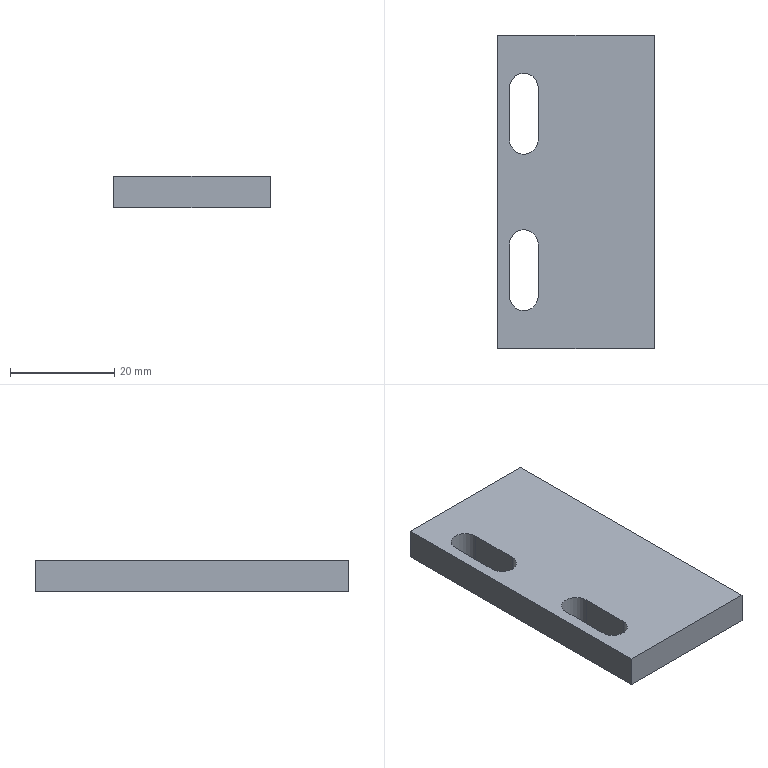Part | STEP file | 0232_208_Plate | 1 solid | 14 faces | box 30 x 60 x 6 mm | volume 9855 mm3 | plane 10 | cylinder 4 | commonest cylinder face diameters 5.5 x4
STEP:
#1=CARTESIAN_POINT('',(0.,0.,0.));
#2=DIRECTION('',(0.,0.,1.));
#3=DIRECTION('',(1.,0.,0.));
#4=AXIS2_PLACEMENT_3D('',#1,#2,#3);
#5=CARTESIAN_POINT('',(-30.,30.,0.));
#6=VERTEX_POINT('',#5);
#7=CARTESIAN_POINT('',(-30.,-30.,0.));
#8=VERTEX_POINT('',#7);
#9=CARTESIAN_POINT('',(-30.,30.,0.));
#10=DIRECTION('',(0.,-1.,0.));
#11=VECTOR('',#10,1.);
#12=LINE('',#9,#11);
#13=CARTESIAN_POINT('',(-30.,30.,6.));
#14=DIRECTION('',(1.,0.,0.));
#15=DIRECTION('',(0.,0.,-1.));
#16=AXIS2_PLACEMENT_3D('',#13,#14,#15);
#17=PLANE('',#16);
#18=CARTESIAN_POINT('',(6.,0.));
#19=DIRECTION('',(0.,-1.));
#20=VECTOR('',#19,1.);
#21=LINE('',#18,#20);
#22=(GEOMETRIC_REPRESENTATION_CONTEXT(2)PARAMETRIC_REPRESENTATION_CONTEXT()REPRESENTATION_CONTEXT('',''));
#23=DEFINITIONAL_REPRESENTATION('',(#21),#22);
#24=PCURVE('',#17,#23);
#25=CARTESIAN_POINT('',(-30.,-30.,0.));
#26=DIRECTION('',(0.,0.,1.));
#27=DIRECTION('',(1.,0.,0.));
#28=AXIS2_PLACEMENT_3D('',#25,#26,#27);
#29=PLANE('',#28);
#30=CARTESIAN_POINT('',(0.,60.));
#31=DIRECTION('',(0.,-1.));
#32=VECTOR('',#31,1.);
#33=LINE('',#30,#32);
#34=(GEOMETRIC_REPRESENTATION_CONTEXT(2)PARAMETRIC_REPRESENTATION_CONTEXT()REPRESENTATION_CONTEXT('',''));
#35=DEFINITIONAL_REPRESENTATION('',(#33),#34);
#36=PCURVE('',#29,#35);
#37=SURFACE_CURVE('',#12,(#24,#36),.PCURVE_S1.);
#38=EDGE_CURVE('',#6,#8,#37,.T.);
#39=ORIENTED_EDGE('',*,*,#38,.T.);
#40=CARTESIAN_POINT('',(-30.,-30.,6.));
#41=VERTEX_POINT('',#40);
#42=CARTESIAN_POINT('',(-30.,-30.,6.));
#43=DIRECTION('',(0.,0.,-1.));
#44=VECTOR('',#43,1.);
#45=LINE('',#42,#44);
#46=CARTESIAN_POINT('',(0.,-60.));
#47=DIRECTION('',(1.,0.));
#48=VECTOR('',#47,1.);
#49=LINE('',#46,#48);
#50=(GEOMETRIC_REPRESENTATION_CONTEXT(2)PARAMETRIC_REPRESENTATION_CONTEXT()REPRESENTATION_CONTEXT('',''));
#51=DEFINITIONAL_REPRESENTATION('',(#49),#50);
#52=PCURVE('',#17,#51);
#53=CARTESIAN_POINT('',(-30.,-30.,6.));
#54=DIRECTION('',(0.,1.,0.));
#55=DIRECTION('',(0.,0.,1.));
#56=AXIS2_PLACEMENT_3D('',#53,#54,#55);
#57=PLANE('',#56);
#58=CARTESIAN_POINT('',(0.,0.));
#59=DIRECTION('',(-1.,0.));
#60=VECTOR('',#59,1.);
#61=LINE('',#58,#60);
#62=(GEOMETRIC_REPRESENTATION_CONTEXT(2)PARAMETRIC_REPRESENTATION_CONTEXT()REPRESENTATION_CONTEXT('',''));
#63=DEFINITIONAL_REPRESENTATION('',(#61),#62);
#64=PCURVE('',#57,#63);
#65=SURFACE_CURVE('',#45,(#52,#64),.PCURVE_S1.);
#66=EDGE_CURVE('',#41,#8,#65,.T.);
#67=ORIENTED_EDGE('',*,*,#66,.F.);
#68=CARTESIAN_POINT('',(-30.,30.,6.));
#69=VERTEX_POINT('',#68);
#70=CARTESIAN_POINT('',(-30.,30.,6.));
#71=DIRECTION('',(0.,-1.,0.));
#72=VECTOR('',#71,1.);
#73=LINE('',#70,#72);
#74=CARTESIAN_POINT('',(0.,0.));
#75=DIRECTION('',(0.,-1.));
#76=VECTOR('',#75,1.);
#77=LINE('',#74,#76);
#78=(GEOMETRIC_REPRESENTATION_CONTEXT(2)PARAMETRIC_REPRESENTATION_CONTEXT()REPRESENTATION_CONTEXT('',''));
#79=DEFINITIONAL_REPRESENTATION('',(#77),#78);
#80=PCURVE('',#17,#79);
#81=CARTESIAN_POINT('',(-30.,-30.,6.));
#82=DIRECTION('',(0.,0.,1.));
#83=DIRECTION('',(1.,0.,0.));
#84=AXIS2_PLACEMENT_3D('',#81,#82,#83);
#85=PLANE('',#84);
#86=CARTESIAN_POINT('',(0.,60.));
#87=DIRECTION('',(0.,-1.));
#88=VECTOR('',#87,1.);
#89=LINE('',#86,#88);
#90=(GEOMETRIC_REPRESENTATION_CONTEXT(2)PARAMETRIC_REPRESENTATION_CONTEXT()REPRESENTATION_CONTEXT('',''));
#91=DEFINITIONAL_REPRESENTATION('',(#89),#90);
#92=PCURVE('',#85,#91);
#93=SURFACE_CURVE('',#73,(#80,#92),.PCURVE_S1.);
#94=EDGE_CURVE('',#69,#41,#93,.T.);
#95=ORIENTED_EDGE('',*,*,#94,.F.);
#96=CARTESIAN_POINT('',(-30.,30.,6.));
#97=DIRECTION('',(0.,0.,-1.));
#98=VECTOR('',#97,1.);
#99=LINE('',#96,#98);
#100=CARTESIAN_POINT('',(0.,0.));
#101=DIRECTION('',(1.,0.));
#102=VECTOR('',#101,1.);
#103=LINE('',#100,#102);
#104=(GEOMETRIC_REPRESENTATION_CONTEXT(2)PARAMETRIC_REPRESENTATION_CONTEXT()REPRESENTATION_CONTEXT('',''));
#105=DEFINITIONAL_REPRESENTATION('',(#103),#104);
#106=PCURVE('',#17,#105);
#107=CARTESIAN_POINT('',(-30.,30.,6.));
#108=DIRECTION('',(0.,-1.,0.));
#109=DIRECTION('',(0.,0.,-1.));
#110=AXIS2_PLACEMENT_3D('',#107,#108,#109);
#111=PLANE('',#110);
#112=CARTESIAN_POINT('',(0.,0.));
#113=DIRECTION('',(1.,0.));
#114=VECTOR('',#113,1.);
#115=LINE('',#112,#114);
#116=(GEOMETRIC_REPRESENTATION_CONTEXT(2)PARAMETRIC_REPRESENTATION_CONTEXT()REPRESENTATION_CONTEXT('',''));
#117=DEFINITIONAL_REPRESENTATION('',(#115),#116);
#118=PCURVE('',#111,#117);
#119=SURFACE_CURVE('',#99,(#106,#118),.PCURVE_S1.);
#120=EDGE_CURVE('',#69,#6,#119,.T.);
#121=ORIENTED_EDGE('',*,*,#120,.T.);
#122=EDGE_LOOP('',(#39,#67,#95,#121));
#123=FACE_BOUND('',#122,.T.);
#124=ADVANCED_FACE('',(#123),#17,.F.);
#125=CARTESIAN_POINT('',(0.,-30.,0.));
#126=VERTEX_POINT('',#125);
#127=CARTESIAN_POINT('',(-30.,-30.,0.));
#128=DIRECTION('',(1.,0.,0.));
#129=VECTOR('',#128,1.);
#130=LINE('',#127,#129);
#131=CARTESIAN_POINT('',(-6.,0.));
#132=DIRECTION('',(0.,1.));
#133=VECTOR('',#132,1.);
#134=LINE('',#131,#133);
#135=(GEOMETRIC_REPRESENTATION_CONTEXT(2)PARAMETRIC_REPRESENTATION_CONTEXT()REPRESENTATION_CONTEXT('',''));
#136=DEFINITIONAL_REPRESENTATION('',(#134),#135);
#137=PCURVE('',#57,#136);
#138=CARTESIAN_POINT('',(0.,0.));
#139=DIRECTION('',(1.,0.));
#140=VECTOR('',#139,1.);
#141=LINE('',#138,#140);
#142=(GEOMETRIC_REPRESENTATION_CONTEXT(2)PARAMETRIC_REPRESENTATION_CONTEXT()REPRESENTATION_CONTEXT('',''));
#143=DEFINITIONAL_REPRESENTATION('',(#141),#142);
#144=PCURVE('',#29,#143);
#145=SURFACE_CURVE('',#130,(#137,#144),.PCURVE_S1.);
#146=EDGE_CURVE('',#8,#126,#145,.T.);
#147=ORIENTED_EDGE('',*,*,#146,.T.);
#148=CARTESIAN_POINT('',(0.,-30.,6.));
#149=VERTEX_POINT('',#148);
#150=CARTESIAN_POINT('',(0.,-30.,6.));
#151=DIRECTION('',(0.,0.,-1.));
#152=VECTOR('',#151,1.);
#153=LINE('',#150,#152);
#154=CARTESIAN_POINT('',(0.,30.));
#155=DIRECTION('',(-1.,0.));
#156=VECTOR('',#155,1.);
#157=LINE('',#154,#156);
#158=(GEOMETRIC_REPRESENTATION_CONTEXT(2)PARAMETRIC_REPRESENTATION_CONTEXT()REPRESENTATION_CONTEXT('',''));
#159=DEFINITIONAL_REPRESENTATION('',(#157),#158);
#160=PCURVE('',#57,#159);
#161=CARTESIAN_POINT('',(0.,30.,6.));
#162=DIRECTION('',(-1.,0.,0.));
#163=DIRECTION('',(0.,0.,1.));
#164=AXIS2_PLACEMENT_3D('',#161,#162,#163);
#165=PLANE('',#164);
#166=CARTESIAN_POINT('',(0.,-60.));
#167=DIRECTION('',(-1.,0.));
#168=VECTOR('',#167,1.);
#169=LINE('',#166,#168);
#170=(GEOMETRIC_REPRESENTATION_CONTEXT(2)PARAMETRIC_REPRESENTATION_CONTEXT()REPRESENTATION_CONTEXT('',''));
#171=DEFINITIONAL_REPRESENTATION('',(#169),#170);
#172=PCURVE('',#165,#171);
#173=SURFACE_CURVE('',#153,(#160,#172),.PCURVE_S1.);
#174=EDGE_CURVE('',#149,#126,#173,.T.);
#175=ORIENTED_EDGE('',*,*,#174,.F.);
#176=CARTESIAN_POINT('',(-30.,-30.,6.));
#177=DIRECTION('',(1.,0.,0.));
#178=VECTOR('',#177,1.);
#179=LINE('',#176,#178);
#180=CARTESIAN_POINT('',(0.,0.));
#181=DIRECTION('',(0.,1.));
#182=VECTOR('',#181,1.);
#183=LINE('',#180,#182);
#184=(GEOMETRIC_REPRESENTATION_CONTEXT(2)PARAMETRIC_REPRESENTATION_CONTEXT()REPRESENTATION_CONTEXT('',''));
#185=DEFINITIONAL_REPRESENTATION('',(#183),#184);
#186=PCURVE('',#57,#185);
#187=CARTESIAN_POINT('',(0.,0.));
#188=DIRECTION('',(1.,0.));
#189=VECTOR('',#188,1.);
#190=LINE('',#187,#189);
#191=(GEOMETRIC_REPRESENTATION_CONTEXT(2)PARAMETRIC_REPRESENTATION_CONTEXT()REPRESENTATION_CONTEXT('',''));
#192=DEFINITIONAL_REPRESENTATION('',(#190),#191);
#193=PCURVE('',#85,#192);
#194=SURFACE_CURVE('',#179,(#186,#193),.PCURVE_S1.);
#195=EDGE_CURVE('',#41,#149,#194,.T.);
#196=ORIENTED_EDGE('',*,*,#195,.F.);
#197=ORIENTED_EDGE('',*,*,#66,.T.);
#198=EDGE_LOOP('',(#147,#175,#196,#197));
#199=FACE_BOUND('',#198,.T.);
#200=ADVANCED_FACE('',(#199),#57,.F.);
#201=CARTESIAN_POINT('',(0.,30.,0.));
#202=VERTEX_POINT('',#201);
#203=CARTESIAN_POINT('',(0.,30.,0.));
#204=DIRECTION('',(0.,1.,0.));
#205=VECTOR('',#204,1.);
#206=LINE('',#203,#205);
#207=CARTESIAN_POINT('',(-6.,0.));
#208=DIRECTION('',(0.,1.));
#209=VECTOR('',#208,1.);
#210=LINE('',#207,#209);
#211=(GEOMETRIC_REPRESENTATION_CONTEXT(2)PARAMETRIC_REPRESENTATION_CONTEXT()REPRESENTATION_CONTEXT('',''));
#212=DEFINITIONAL_REPRESENTATION('',(#210),#211);
#213=PCURVE('',#165,#212);
#214=CARTESIAN_POINT('',(30.,60.));
#215=DIRECTION('',(0.,1.));
#216=VECTOR('',#215,1.);
#217=LINE('',#214,#216);
#218=(GEOMETRIC_REPRESENTATION_CONTEXT(2)PARAMETRIC_REPRESENTATION_CONTEXT()REPRESENTATION_CONTEXT('',''));
#219=DEFINITIONAL_REPRESENTATION('',(#217),#218);
#220=PCURVE('',#29,#219);
#221=SURFACE_CURVE('',#206,(#213,#220),.PCURVE_S1.);
#222=EDGE_CURVE('',#126,#202,#221,.T.);
#223=ORIENTED_EDGE('',*,*,#222,.T.);
#224=CARTESIAN_POINT('',(0.,30.,6.));
#225=VERTEX_POINT('',#224);
#226=CARTESIAN_POINT('',(0.,30.,6.));
#227=DIRECTION('',(0.,0.,-1.));
#228=VECTOR('',#227,1.);
#229=LINE('',#226,#228);
#230=CARTESIAN_POINT('',(0.,0.));
#231=DIRECTION('',(-1.,0.));
#232=VECTOR('',#231,1.);
#233=LINE('',#230,#232);
#234=(GEOMETRIC_REPRESENTATION_CONTEXT(2)PARAMETRIC_REPRESENTATION_CONTEXT()REPRESENTATION_CONTEXT('',''));
#235=DEFINITIONAL_REPRESENTATION('',(#233),#234);
#236=PCURVE('',#165,#235);
#237=CARTESIAN_POINT('',(0.,30.));
#238=DIRECTION('',(1.,0.));
#239=VECTOR('',#238,1.);
#240=LINE('',#237,#239);
#241=(GEOMETRIC_REPRESENTATION_CONTEXT(2)PARAMETRIC_REPRESENTATION_CONTEXT()REPRESENTATION_CONTEXT('',''));
#242=DEFINITIONAL_REPRESENTATION('',(#240),#241);
#243=PCURVE('',#111,#242);
#244=SURFACE_CURVE('',#229,(#236,#243),.PCURVE_S1.);
#245=EDGE_CURVE('',#225,#202,#244,.T.);
#246=ORIENTED_EDGE('',*,*,#245,.F.);
#247=CARTESIAN_POINT('',(0.,30.,6.));
#248=DIRECTION('',(0.,1.,0.));
#249=VECTOR('',#248,1.);
#250=LINE('',#247,#249);
#251=CARTESIAN_POINT('',(0.,0.));
#252=DIRECTION('',(0.,1.));
#253=VECTOR('',#252,1.);
#254=LINE('',#251,#253);
#255=(GEOMETRIC_REPRESENTATION_CONTEXT(2)PARAMETRIC_REPRESENTATION_CONTEXT()REPRESENTATION_CONTEXT('',''));
#256=DEFINITIONAL_REPRESENTATION('',(#254),#255);
#257=PCURVE('',#165,#256);
#258=CARTESIAN_POINT('',(30.,60.));
#259=DIRECTION('',(0.,1.));
#260=VECTOR('',#259,1.);
#261=LINE('',#258,#260);
#262=(GEOMETRIC_REPRESENTATION_CONTEXT(2)PARAMETRIC_REPRESENTATION_CONTEXT()REPRESENTATION_CONTEXT('',''));
#263=DEFINITIONAL_REPRESENTATION('',(#261),#262);
#264=PCURVE('',#85,#263);
#265=SURFACE_CURVE('',#250,(#257,#264),.PCURVE_S1.);
#266=EDGE_CURVE('',#149,#225,#265,.T.);
#267=ORIENTED_EDGE('',*,*,#266,.F.);
#268=ORIENTED_EDGE('',*,*,#174,.T.);
#269=EDGE_LOOP('',(#223,#246,#267,#268));
#270=FACE_BOUND('',#269,.T.);
#271=ADVANCED_FACE('',(#270),#165,.F.);
#272=CARTESIAN_POINT('',(-30.,30.,0.));
#273=DIRECTION('',(-1.,0.,0.));
#274=VECTOR('',#273,1.);
#275=LINE('',#272,#274);
#276=CARTESIAN_POINT('',(6.,0.));
#277=DIRECTION('',(0.,-1.));
#278=VECTOR('',#277,1.);
#279=LINE('',#276,#278);
#280=(GEOMETRIC_REPRESENTATION_CONTEXT(2)PARAMETRIC_REPRESENTATION_CONTEXT()REPRESENTATION_CONTEXT('',''));
#281=DEFINITIONAL_REPRESENTATION('',(#279),#280);
#282=PCURVE('',#111,#281);
#283=CARTESIAN_POINT('',(0.,60.));
#284=DIRECTION('',(-1.,0.));
#285=VECTOR('',#284,1.);
#286=LINE('',#283,#285);
#287=(GEOMETRIC_REPRESENTATION_CONTEXT(2)PARAMETRIC_REPRESENTATION_CONTEXT()REPRESENTATION_CONTEXT('',''));
#288=DEFINITIONAL_REPRESENTATION('',(#286),#287);
#289=PCURVE('',#29,#288);
#290=SURFACE_CURVE('',#275,(#282,#289),.PCURVE_S1.);
#291=EDGE_CURVE('',#202,#6,#290,.T.);
#292=ORIENTED_EDGE('',*,*,#291,.T.);
#293=ORIENTED_EDGE('',*,*,#120,.F.);
#294=CARTESIAN_POINT('',(-30.,30.,6.));
#295=DIRECTION('',(-1.,0.,0.));
#296=VECTOR('',#295,1.);
#297=LINE('',#294,#296);
#298=CARTESIAN_POINT('',(0.,0.));
#299=DIRECTION('',(0.,-1.));
#300=VECTOR('',#299,1.);
#301=LINE('',#298,#300);
#302=(GEOMETRIC_REPRESENTATION_CONTEXT(2)PARAMETRIC_REPRESENTATION_CONTEXT()REPRESENTATION_CONTEXT('',''));
#303=DEFINITIONAL_REPRESENTATION('',(#301),#302);
#304=PCURVE('',#111,#303);
#305=CARTESIAN_POINT('',(0.,60.));
#306=DIRECTION('',(-1.,0.));
#307=VECTOR('',#306,1.);
#308=LINE('',#305,#307);
#309=(GEOMETRIC_REPRESENTATION_CONTEXT(2)PARAMETRIC_REPRESENTATION_CONTEXT()REPRESENTATION_CONTEXT('',''));
#310=DEFINITIONAL_REPRESENTATION('',(#308),#309);
#311=PCURVE('',#85,#310);
#312=SURFACE_CURVE('',#297,(#304,#311),.PCURVE_S1.);
#313=EDGE_CURVE('',#225,#69,#312,.T.);
#314=ORIENTED_EDGE('',*,*,#313,.F.);
#315=ORIENTED_EDGE('',*,*,#245,.T.);
#316=EDGE_LOOP('',(#292,#293,#314,#315));
#317=FACE_BOUND('',#316,.T.);
#318=ADVANCED_FACE('',(#317),#111,.F.);
#319=CARTESIAN_POINT('',(-27.75,-20.,6.));
#320=VERTEX_POINT('',#319);
#321=CARTESIAN_POINT('',(-22.25,-20.,6.));
#322=VERTEX_POINT('',#321);
#323=CARTESIAN_POINT('',(-25.,-20.,6.));
#324=DIRECTION('',(0.,0.,1.));
#325=DIRECTION('',(-1.,0.,0.));
#326=AXIS2_PLACEMENT_3D('',#323,#324,#325);
#327=CIRCLE('',#326,2.75);
#328=CARTESIAN_POINT('',(5.,10.));
#329=DIRECTION('',(-1.,0.));
#330=AXIS2_PLACEMENT_2D('',#328,#329);
#331=CIRCLE('',#330,2.75);
#332=(GEOMETRIC_REPRESENTATION_CONTEXT(2)PARAMETRIC_REPRESENTATION_CONTEXT()REPRESENTATION_CONTEXT('',''));
#333=DEFINITIONAL_REPRESENTATION('',(#331),#332);
#334=PCURVE('',#85,#333);
#335=CARTESIAN_POINT('',(-25.,-20.,0.));
#336=DIRECTION('',(0.,0.,1.));
#337=DIRECTION('',(1.,0.,0.));
#338=AXIS2_PLACEMENT_3D('',#335,#336,#337);
#339=CYLINDRICAL_SURFACE('',#338,2.75);
#340=CARTESIAN_POINT('',(3.142,6.));
#341=DIRECTION('',(1.,0.));
#342=VECTOR('',#341,1.);
#343=LINE('',#340,#342);
#344=(GEOMETRIC_REPRESENTATION_CONTEXT(2)PARAMETRIC_REPRESENTATION_CONTEXT()REPRESENTATION_CONTEXT('',''));
#345=DEFINITIONAL_REPRESENTATION('',(#343),#344);
#346=PCURVE('',#339,#345);
#347=SURFACE_CURVE('',#327,(#334,#346),.PCURVE_S1.);
#348=EDGE_CURVE('',#320,#322,#347,.T.);
#349=ORIENTED_EDGE('',*,*,#348,.F.);
#350=CARTESIAN_POINT('',(-27.75,-10.,6.));
#351=VERTEX_POINT('',#350);
#352=CARTESIAN_POINT('',(-27.75,-20.,6.));
#353=DIRECTION('',(0.,-1.,0.));
#354=VECTOR('',#353,1.);
#355=LINE('',#352,#354);
#356=CARTESIAN_POINT('',(2.25,10.));
#357=DIRECTION('',(0.,-1.));
#358=VECTOR('',#357,1.);
#359=LINE('',#356,#358);
#360=(GEOMETRIC_REPRESENTATION_CONTEXT(2)PARAMETRIC_REPRESENTATION_CONTEXT()REPRESENTATION_CONTEXT('',''));
#361=DEFINITIONAL_REPRESENTATION('',(#359),#360);
#362=PCURVE('',#85,#361);
#363=CARTESIAN_POINT('',(-27.75,-20.,0.));
#364=DIRECTION('',(-1.,0.,0.));
#365=DIRECTION('',(0.,0.,1.));
#366=AXIS2_PLACEMENT_3D('',#363,#364,#365);
#367=PLANE('',#366);
#368=CARTESIAN_POINT('',(6.,0.));
#369=DIRECTION('',(0.,-1.));
#370=VECTOR('',#369,1.);
#371=LINE('',#368,#370);
#372=(GEOMETRIC_REPRESENTATION_CONTEXT(2)PARAMETRIC_REPRESENTATION_CONTEXT()REPRESENTATION_CONTEXT('',''));
#373=DEFINITIONAL_REPRESENTATION('',(#371),#372);
#374=PCURVE('',#367,#373);
#375=SURFACE_CURVE('',#355,(#362,#374),.PCURVE_S1.);
#376=EDGE_CURVE('',#351,#320,#375,.T.);
#377=ORIENTED_EDGE('',*,*,#376,.F.);
#378=CARTESIAN_POINT('',(-22.25,-10.,6.));
#379=VERTEX_POINT('',#378);
#380=CARTESIAN_POINT('',(-25.,-10.,6.));
#381=DIRECTION('',(0.,0.,1.));
#382=DIRECTION('',(-1.,0.,0.));
#383=AXIS2_PLACEMENT_3D('',#380,#381,#382);
#384=CIRCLE('',#383,2.75);
#385=CARTESIAN_POINT('',(5.,20.));
#386=DIRECTION('',(-1.,0.));
#387=AXIS2_PLACEMENT_2D('',#385,#386);
#388=CIRCLE('',#387,2.75);
#389=(GEOMETRIC_REPRESENTATION_CONTEXT(2)PARAMETRIC_REPRESENTATION_CONTEXT()REPRESENTATION_CONTEXT('',''));
#390=DEFINITIONAL_REPRESENTATION('',(#388),#389);
#391=PCURVE('',#85,#390);
#392=CARTESIAN_POINT('',(-25.,-10.,0.));
#393=DIRECTION('',(0.,0.,1.));
#394=DIRECTION('',(1.,0.,0.));
#395=AXIS2_PLACEMENT_3D('',#392,#393,#394);
#396=CYLINDRICAL_SURFACE('',#395,2.75);
#397=CARTESIAN_POINT('',(-3.142,6.));
#398=DIRECTION('',(1.,0.));
#399=VECTOR('',#398,1.);
#400=LINE('',#397,#399);
#401=(GEOMETRIC_REPRESENTATION_CONTEXT(2)PARAMETRIC_REPRESENTATION_CONTEXT()REPRESENTATION_CONTEXT('',''));
#402=DEFINITIONAL_REPRESENTATION('',(#400),#401);
#403=PCURVE('',#396,#402);
#404=SURFACE_CURVE('',#384,(#391,#403),.PCURVE_S1.);
#405=EDGE_CURVE('',#379,#351,#404,.T.);
#406=ORIENTED_EDGE('',*,*,#405,.F.);
#407=CARTESIAN_POINT('',(-22.25,-20.,6.));
#408=DIRECTION('',(0.,1.,0.));
#409=VECTOR('',#408,1.);
#410=LINE('',#407,#409);
#411=CARTESIAN_POINT('',(7.75,10.));
#412=DIRECTION('',(0.,1.));
#413=VECTOR('',#412,1.);
#414=LINE('',#411,#413);
#415=(GEOMETRIC_REPRESENTATION_CONTEXT(2)PARAMETRIC_REPRESENTATION_CONTEXT()REPRESENTATION_CONTEXT('',''));
#416=DEFINITIONAL_REPRESENTATION('',(#414),#415);
#417=PCURVE('',#85,#416);
#418=CARTESIAN_POINT('',(-22.25,-20.,0.));
#419=DIRECTION('',(1.,0.,0.));
#420=DIRECTION('',(0.,0.,-1.));
#421=AXIS2_PLACEMENT_3D('',#418,#419,#420);
#422=PLANE('',#421);
#423=CARTESIAN_POINT('',(-6.,0.));
#424=DIRECTION('',(0.,1.));
#425=VECTOR('',#424,1.);
#426=LINE('',#423,#425);
#427=(GEOMETRIC_REPRESENTATION_CONTEXT(2)PARAMETRIC_REPRESENTATION_CONTEXT()REPRESENTATION_CONTEXT('',''));
#428=DEFINITIONAL_REPRESENTATION('',(#426),#427);
#429=PCURVE('',#422,#428);
#430=SURFACE_CURVE('',#410,(#417,#429),.PCURVE_S1.);
#431=EDGE_CURVE('',#322,#379,#430,.T.);
#432=ORIENTED_EDGE('',*,*,#431,.F.);
#433=EDGE_LOOP('',(#349,#377,#406,#432));
#434=FACE_BOUND('',#433,.T.);
#435=CARTESIAN_POINT('',(-22.25,20.,6.));
#436=VERTEX_POINT('',#435);
#437=CARTESIAN_POINT('',(-27.75,20.,6.));
#438=VERTEX_POINT('',#437);
#439=CARTESIAN_POINT('',(-25.,20.,6.));
#440=DIRECTION('',(0.,0.,1.));
#441=DIRECTION('',(1.,0.,0.));
#442=AXIS2_PLACEMENT_3D('',#439,#440,#441);
#443=CIRCLE('',#442,2.75);
#444=CARTESIAN_POINT('',(5.,50.));
#445=DIRECTION('',(1.,0.));
#446=AXIS2_PLACEMENT_2D('',#444,#445);
#447=CIRCLE('',#446,2.75);
#448=(GEOMETRIC_REPRESENTATION_CONTEXT(2)PARAMETRIC_REPRESENTATION_CONTEXT()REPRESENTATION_CONTEXT('',''));
#449=DEFINITIONAL_REPRESENTATION('',(#447),#448);
#450=PCURVE('',#85,#449);
#451=CARTESIAN_POINT('',(-25.,20.,0.));
#452=DIRECTION('',(0.,0.,1.));
#453=DIRECTION('',(1.,0.,0.));
#454=AXIS2_PLACEMENT_3D('',#451,#452,#453);
#455=CYLINDRICAL_SURFACE('',#454,2.75);
#456=CARTESIAN_POINT('',(0.,6.));
#457=DIRECTION('',(1.,0.));
#458=VECTOR('',#457,1.);
#459=LINE('',#456,#458);
#460=(GEOMETRIC_REPRESENTATION_CONTEXT(2)PARAMETRIC_REPRESENTATION_CONTEXT()REPRESENTATION_CONTEXT('',''));
#461=DEFINITIONAL_REPRESENTATION('',(#459),#460);
#462=PCURVE('',#455,#461);
#463=SURFACE_CURVE('',#443,(#450,#462),.PCURVE_S1.);
#464=EDGE_CURVE('',#436,#438,#463,.T.);
#465=ORIENTED_EDGE('',*,*,#464,.F.);
#466=CARTESIAN_POINT('',(-22.25,10.,6.));
#467=VERTEX_POINT('',#466);
#468=CARTESIAN_POINT('',(-22.25,20.,6.));
#469=DIRECTION('',(0.,1.,0.));
#470=VECTOR('',#469,1.);
#471=LINE('',#468,#470);
#472=CARTESIAN_POINT('',(7.75,50.));
#473=DIRECTION('',(0.,1.));
#474=VECTOR('',#473,1.);
#475=LINE('',#472,#474);
#476=(GEOMETRIC_REPRESENTATION_CONTEXT(2)PARAMETRIC_REPRESENTATION_CONTEXT()REPRESENTATION_CONTEXT('',''));
#477=DEFINITIONAL_REPRESENTATION('',(#475),#476);
#478=PCURVE('',#85,#477);
#479=CARTESIAN_POINT('',(-22.25,20.,0.));
#480=DIRECTION('',(1.,0.,0.));
#481=DIRECTION('',(0.,0.,-1.));
#482=AXIS2_PLACEMENT_3D('',#479,#480,#481);
#483=PLANE('',#482);
#484=CARTESIAN_POINT('',(-6.,0.));
#485=DIRECTION('',(0.,1.));
#486=VECTOR('',#485,1.);
#487=LINE('',#484,#486);
#488=(GEOMETRIC_REPRESENTATION_CONTEXT(2)PARAMETRIC_REPRESENTATION_CONTEXT()REPRESENTATION_CONTEXT('',''));
#489=DEFINITIONAL_REPRESENTATION('',(#487),#488);
#490=PCURVE('',#483,#489);
#491=SURFACE_CURVE('',#471,(#478,#490),.PCURVE_S1.);
#492=EDGE_CURVE('',#467,#436,#491,.T.);
#493=ORIENTED_EDGE('',*,*,#492,.F.);
#494=CARTESIAN_POINT('',(-27.75,10.,6.));
#495=VERTEX_POINT('',#494);
#496=CARTESIAN_POINT('',(-25.,10.,6.));
#497=DIRECTION('',(0.,0.,1.));
#498=DIRECTION('',(1.,0.,0.));
#499=AXIS2_PLACEMENT_3D('',#496,#497,#498);
#500=CIRCLE('',#499,2.75);
#501=CARTESIAN_POINT('',(5.,40.));
#502=DIRECTION('',(1.,0.));
#503=AXIS2_PLACEMENT_2D('',#501,#502);
#504=CIRCLE('',#503,2.75);
#505=(GEOMETRIC_REPRESENTATION_CONTEXT(2)PARAMETRIC_REPRESENTATION_CONTEXT()REPRESENTATION_CONTEXT('',''));
#506=DEFINITIONAL_REPRESENTATION('',(#504),#505);
#507=PCURVE('',#85,#506);
#508=CARTESIAN_POINT('',(-25.,10.,0.));
#509=DIRECTION('',(0.,0.,1.));
#510=DIRECTION('',(1.,0.,0.));
#511=AXIS2_PLACEMENT_3D('',#508,#509,#510);
#512=CYLINDRICAL_SURFACE('',#511,2.75);
#513=CARTESIAN_POINT('',(0.,6.));
#514=DIRECTION('',(1.,0.));
#515=VECTOR('',#514,1.);
#516=LINE('',#513,#515);
#517=(GEOMETRIC_REPRESENTATION_CONTEXT(2)PARAMETRIC_REPRESENTATION_CONTEXT()REPRESENTATION_CONTEXT('',''));
#518=DEFINITIONAL_REPRESENTATION('',(#516),#517);
#519=PCURVE('',#512,#518);
#520=SURFACE_CURVE('',#500,(#507,#519),.PCURVE_S1.);
#521=EDGE_CURVE('',#495,#467,#520,.T.);
#522=ORIENTED_EDGE('',*,*,#521,.F.);
#523=CARTESIAN_POINT('',(-27.75,20.,6.));
#524=DIRECTION('',(0.,-1.,0.));
#525=VECTOR('',#524,1.);
#526=LINE('',#523,#525);
#527=CARTESIAN_POINT('',(2.25,50.));
#528=DIRECTION('',(0.,-1.));
#529=VECTOR('',#528,1.);
#530=LINE('',#527,#529);
#531=(GEOMETRIC_REPRESENTATION_CONTEXT(2)PARAMETRIC_REPRESENTATION_CONTEXT()REPRESENTATION_CONTEXT('',''));
#532=DEFINITIONAL_REPRESENTATION('',(#530),#531);
#533=PCURVE('',#85,#532);
#534=CARTESIAN_POINT('',(-27.75,20.,0.));
#535=DIRECTION('',(-1.,0.,0.));
#536=DIRECTION('',(0.,0.,1.));
#537=AXIS2_PLACEMENT_3D('',#534,#535,#536);
#538=PLANE('',#537);
#539=CARTESIAN_POINT('',(6.,0.));
#540=DIRECTION('',(0.,-1.));
#541=VECTOR('',#540,1.);
#542=LINE('',#539,#541);
#543=(GEOMETRIC_REPRESENTATION_CONTEXT(2)PARAMETRIC_REPRESENTATION_CONTEXT()REPRESENTATION_CONTEXT('',''));
#544=DEFINITIONAL_REPRESENTATION('',(#542),#543);
#545=PCURVE('',#538,#544);
#546=SURFACE_CURVE('',#526,(#533,#545),.PCURVE_S1.);
#547=EDGE_CURVE('',#438,#495,#546,.T.);
#548=ORIENTED_EDGE('',*,*,#547,.F.);
#549=EDGE_LOOP('',(#465,#493,#522,#548));
#550=FACE_BOUND('',#549,.T.);
#551=ORIENTED_EDGE('',*,*,#94,.T.);
#552=ORIENTED_EDGE('',*,*,#195,.T.);
#553=ORIENTED_EDGE('',*,*,#266,.T.);
#554=ORIENTED_EDGE('',*,*,#313,.T.);
#555=EDGE_LOOP('',(#551,#552,#553,#554));
#556=FACE_BOUND('',#555,.T.);
#557=ADVANCED_FACE('',(#434,#550,#556),#85,.T.);
#558=CARTESIAN_POINT('',(-27.75,-10.,0.));
#559=VERTEX_POINT('',#558);
#560=CARTESIAN_POINT('',(-27.75,-20.,0.));
#561=VERTEX_POINT('',#560);
#562=CARTESIAN_POINT('',(-27.75,-20.,0.));
#563=DIRECTION('',(0.,-1.,0.));
#564=VECTOR('',#563,1.);
#565=LINE('',#562,#564);
#566=CARTESIAN_POINT('',(2.25,10.));
#567=DIRECTION('',(0.,-1.));
#568=VECTOR('',#567,1.);
#569=LINE('',#566,#568);
#570=(GEOMETRIC_REPRESENTATION_CONTEXT(2)PARAMETRIC_REPRESENTATION_CONTEXT()REPRESENTATION_CONTEXT('',''));
#571=DEFINITIONAL_REPRESENTATION('',(#569),#570);
#572=PCURVE('',#29,#571);
#573=CARTESIAN_POINT('',(0.,0.));
#574=DIRECTION('',(0.,-1.));
#575=VECTOR('',#574,1.);
#576=LINE('',#573,#575);
#577=(GEOMETRIC_REPRESENTATION_CONTEXT(2)PARAMETRIC_REPRESENTATION_CONTEXT()REPRESENTATION_CONTEXT('',''));
#578=DEFINITIONAL_REPRESENTATION('',(#576),#577);
#579=PCURVE('',#367,#578);
#580=SURFACE_CURVE('',#565,(#572,#579),.PCURVE_S1.);
#581=EDGE_CURVE('',#559,#561,#580,.T.);
#582=ORIENTED_EDGE('',*,*,#581,.T.);
#583=CARTESIAN_POINT('',(-22.25,-20.,0.));
#584=VERTEX_POINT('',#583);
#585=CARTESIAN_POINT('',(-25.,-20.,0.));
#586=DIRECTION('',(0.,0.,1.));
#587=DIRECTION('',(-1.,0.,0.));
#588=AXIS2_PLACEMENT_3D('',#585,#586,#587);
#589=CIRCLE('',#588,2.75);
#590=CARTESIAN_POINT('',(5.,10.));
#591=DIRECTION('',(-1.,0.));
#592=AXIS2_PLACEMENT_2D('',#590,#591);
#593=CIRCLE('',#592,2.75);
#594=(GEOMETRIC_REPRESENTATION_CONTEXT(2)PARAMETRIC_REPRESENTATION_CONTEXT()REPRESENTATION_CONTEXT('',''));
#595=DEFINITIONAL_REPRESENTATION('',(#593),#594);
#596=PCURVE('',#29,#595);
#597=CARTESIAN_POINT('',(3.142,0.));
#598=DIRECTION('',(1.,0.));
#599=VECTOR('',#598,1.);
#600=LINE('',#597,#599);
#601=(GEOMETRIC_REPRESENTATION_CONTEXT(2)PARAMETRIC_REPRESENTATION_CONTEXT()REPRESENTATION_CONTEXT('',''));
#602=DEFINITIONAL_REPRESENTATION('',(#600),#601);
#603=PCURVE('',#339,#602);
#604=SURFACE_CURVE('',#589,(#596,#603),.PCURVE_S1.);
#605=EDGE_CURVE('',#561,#584,#604,.T.);
#606=ORIENTED_EDGE('',*,*,#605,.T.);
#607=CARTESIAN_POINT('',(-22.25,-10.,0.));
#608=VERTEX_POINT('',#607);
#609=CARTESIAN_POINT('',(-22.25,-20.,0.));
#610=DIRECTION('',(0.,1.,0.));
#611=VECTOR('',#610,1.);
#612=LINE('',#609,#611);
#613=CARTESIAN_POINT('',(7.75,10.));
#614=DIRECTION('',(0.,1.));
#615=VECTOR('',#614,1.);
#616=LINE('',#613,#615);
#617=(GEOMETRIC_REPRESENTATION_CONTEXT(2)PARAMETRIC_REPRESENTATION_CONTEXT()REPRESENTATION_CONTEXT('',''));
#618=DEFINITIONAL_REPRESENTATION('',(#616),#617);
#619=PCURVE('',#29,#618);
#620=CARTESIAN_POINT('',(0.,0.));
#621=DIRECTION('',(0.,1.));
#622=VECTOR('',#621,1.);
#623=LINE('',#620,#622);
#624=(GEOMETRIC_REPRESENTATION_CONTEXT(2)PARAMETRIC_REPRESENTATION_CONTEXT()REPRESENTATION_CONTEXT('',''));
#625=DEFINITIONAL_REPRESENTATION('',(#623),#624);
#626=PCURVE('',#422,#625);
#627=SURFACE_CURVE('',#612,(#619,#626),.PCURVE_S1.);
#628=EDGE_CURVE('',#584,#608,#627,.T.);
#629=ORIENTED_EDGE('',*,*,#628,.T.);
#630=CARTESIAN_POINT('',(-25.,-10.,0.));
#631=DIRECTION('',(0.,0.,1.));
#632=DIRECTION('',(-1.,0.,0.));
#633=AXIS2_PLACEMENT_3D('',#630,#631,#632);
#634=CIRCLE('',#633,2.75);
#635=CARTESIAN_POINT('',(5.,20.));
#636=DIRECTION('',(-1.,0.));
#637=AXIS2_PLACEMENT_2D('',#635,#636);
#638=CIRCLE('',#637,2.75);
#639=(GEOMETRIC_REPRESENTATION_CONTEXT(2)PARAMETRIC_REPRESENTATION_CONTEXT()REPRESENTATION_CONTEXT('',''));
#640=DEFINITIONAL_REPRESENTATION('',(#638),#639);
#641=PCURVE('',#29,#640);
#642=CARTESIAN_POINT('',(-3.142,0.));
#643=DIRECTION('',(1.,0.));
#644=VECTOR('',#643,1.);
#645=LINE('',#642,#644);
#646=(GEOMETRIC_REPRESENTATION_CONTEXT(2)PARAMETRIC_REPRESENTATION_CONTEXT()REPRESENTATION_CONTEXT('',''));
#647=DEFINITIONAL_REPRESENTATION('',(#645),#646);
#648=PCURVE('',#396,#647);
#649=SURFACE_CURVE('',#634,(#641,#648),.PCURVE_S1.);
#650=EDGE_CURVE('',#608,#559,#649,.T.);
#651=ORIENTED_EDGE('',*,*,#650,.T.);
#652=EDGE_LOOP('',(#582,#606,#629,#651));
#653=FACE_BOUND('',#652,.T.);
#654=CARTESIAN_POINT('',(-22.25,10.,0.));
#655=VERTEX_POINT('',#654);
#656=CARTESIAN_POINT('',(-22.25,20.,0.));
#657=VERTEX_POINT('',#656);
#658=CARTESIAN_POINT('',(-22.25,20.,0.));
#659=DIRECTION('',(0.,1.,0.));
#660=VECTOR('',#659,1.);
#661=LINE('',#658,#660);
#662=CARTESIAN_POINT('',(7.75,50.));
#663=DIRECTION('',(0.,1.));
#664=VECTOR('',#663,1.);
#665=LINE('',#662,#664);
#666=(GEOMETRIC_REPRESENTATION_CONTEXT(2)PARAMETRIC_REPRESENTATION_CONTEXT()REPRESENTATION_CONTEXT('',''));
#667=DEFINITIONAL_REPRESENTATION('',(#665),#666);
#668=PCURVE('',#29,#667);
#669=CARTESIAN_POINT('',(0.,0.));
#670=DIRECTION('',(0.,1.));
#671=VECTOR('',#670,1.);
#672=LINE('',#669,#671);
#673=(GEOMETRIC_REPRESENTATION_CONTEXT(2)PARAMETRIC_REPRESENTATION_CONTEXT()REPRESENTATION_CONTEXT('',''));
#674=DEFINITIONAL_REPRESENTATION('',(#672),#673);
#675=PCURVE('',#483,#674);
#676=SURFACE_CURVE('',#661,(#668,#675),.PCURVE_S1.);
#677=EDGE_CURVE('',#655,#657,#676,.T.);
#678=ORIENTED_EDGE('',*,*,#677,.T.);
#679=CARTESIAN_POINT('',(-27.75,20.,0.));
#680=VERTEX_POINT('',#679);
#681=CARTESIAN_POINT('',(-25.,20.,0.));
#682=DIRECTION('',(0.,0.,1.));
#683=DIRECTION('',(1.,0.,0.));
#684=AXIS2_PLACEMENT_3D('',#681,#682,#683);
#685=CIRCLE('',#684,2.75);
#686=CARTESIAN_POINT('',(5.,50.));
#687=DIRECTION('',(1.,0.));
#688=AXIS2_PLACEMENT_2D('',#686,#687);
#689=CIRCLE('',#688,2.75);
#690=(GEOMETRIC_REPRESENTATION_CONTEXT(2)PARAMETRIC_REPRESENTATION_CONTEXT()REPRESENTATION_CONTEXT('',''));
#691=DEFINITIONAL_REPRESENTATION('',(#689),#690);
#692=PCURVE('',#29,#691);
#693=CARTESIAN_POINT('',(0.,0.));
#694=DIRECTION('',(1.,0.));
#695=VECTOR('',#694,1.);
#696=LINE('',#693,#695);
#697=(GEOMETRIC_REPRESENTATION_CONTEXT(2)PARAMETRIC_REPRESENTATION_CONTEXT()REPRESENTATION_CONTEXT('',''));
#698=DEFINITIONAL_REPRESENTATION('',(#696),#697);
#699=PCURVE('',#455,#698);
#700=SURFACE_CURVE('',#685,(#692,#699),.PCURVE_S1.);
#701=EDGE_CURVE('',#657,#680,#700,.T.);
#702=ORIENTED_EDGE('',*,*,#701,.T.);
#703=CARTESIAN_POINT('',(-27.75,10.,0.));
#704=VERTEX_POINT('',#703);
#705=CARTESIAN_POINT('',(-27.75,20.,0.));
#706=DIRECTION('',(0.,-1.,0.));
#707=VECTOR('',#706,1.);
#708=LINE('',#705,#707);
#709=CARTESIAN_POINT('',(2.25,50.));
#710=DIRECTION('',(0.,-1.));
#711=VECTOR('',#710,1.);
#712=LINE('',#709,#711);
#713=(GEOMETRIC_REPRESENTATION_CONTEXT(2)PARAMETRIC_REPRESENTATION_CONTEXT()REPRESENTATION_CONTEXT('',''));
#714=DEFINITIONAL_REPRESENTATION('',(#712),#713);
#715=PCURVE('',#29,#714);
#716=CARTESIAN_POINT('',(0.,0.));
#717=DIRECTION('',(0.,-1.));
#718=VECTOR('',#717,1.);
#719=LINE('',#716,#718);
#720=(GEOMETRIC_REPRESENTATION_CONTEXT(2)PARAMETRIC_REPRESENTATION_CONTEXT()REPRESENTATION_CONTEXT('',''));
#721=DEFINITIONAL_REPRESENTATION('',(#719),#720);
#722=PCURVE('',#538,#721);
#723=SURFACE_CURVE('',#708,(#715,#722),.PCURVE_S1.);
#724=EDGE_CURVE('',#680,#704,#723,.T.);
#725=ORIENTED_EDGE('',*,*,#724,.T.);
#726=CARTESIAN_POINT('',(-25.,10.,0.));
#727=DIRECTION('',(0.,0.,1.));
#728=DIRECTION('',(1.,0.,0.));
#729=AXIS2_PLACEMENT_3D('',#726,#727,#728);
#730=CIRCLE('',#729,2.75);
#731=CARTESIAN_POINT('',(5.,40.));
#732=DIRECTION('',(1.,0.));
#733=AXIS2_PLACEMENT_2D('',#731,#732);
#734=CIRCLE('',#733,2.75);
#735=(GEOMETRIC_REPRESENTATION_CONTEXT(2)PARAMETRIC_REPRESENTATION_CONTEXT()REPRESENTATION_CONTEXT('',''));
#736=DEFINITIONAL_REPRESENTATION('',(#734),#735);
#737=PCURVE('',#29,#736);
#738=CARTESIAN_POINT('',(0.,0.));
#739=DIRECTION('',(1.,0.));
#740=VECTOR('',#739,1.);
#741=LINE('',#738,#740);
#742=(GEOMETRIC_REPRESENTATION_CONTEXT(2)PARAMETRIC_REPRESENTATION_CONTEXT()REPRESENTATION_CONTEXT('',''));
#743=DEFINITIONAL_REPRESENTATION('',(#741),#742);
#744=PCURVE('',#512,#743);
#745=SURFACE_CURVE('',#730,(#737,#744),.PCURVE_S1.);
#746=EDGE_CURVE('',#704,#655,#745,.T.);
#747=ORIENTED_EDGE('',*,*,#746,.T.);
#748=EDGE_LOOP('',(#678,#702,#725,#747));
#749=FACE_BOUND('',#748,.T.);
#750=ORIENTED_EDGE('',*,*,#38,.F.);
#751=ORIENTED_EDGE('',*,*,#291,.F.);
#752=ORIENTED_EDGE('',*,*,#222,.F.);
#753=ORIENTED_EDGE('',*,*,#146,.F.);
#754=EDGE_LOOP('',(#750,#751,#752,#753));
#755=FACE_BOUND('',#754,.T.);
#756=ADVANCED_FACE('',(#653,#749,#755),#29,.F.);
#757=CARTESIAN_POINT('',(-22.25,20.,0.));
#758=DIRECTION('',(0.,0.,1.));
#759=VECTOR('',#758,1.);
#760=LINE('',#757,#759);
#761=CARTESIAN_POINT('',(0.,0.));
#762=DIRECTION('',(0.,1.));
#763=VECTOR('',#762,1.);
#764=LINE('',#761,#763);
#765=(GEOMETRIC_REPRESENTATION_CONTEXT(2)PARAMETRIC_REPRESENTATION_CONTEXT()REPRESENTATION_CONTEXT('',''));
#766=DEFINITIONAL_REPRESENTATION('',(#764),#765);
#767=PCURVE('',#455,#766);
#768=CARTESIAN_POINT('',(0.,0.));
#769=DIRECTION('',(-1.,0.));
#770=VECTOR('',#769,1.);
#771=LINE('',#768,#770);
#772=(GEOMETRIC_REPRESENTATION_CONTEXT(2)PARAMETRIC_REPRESENTATION_CONTEXT()REPRESENTATION_CONTEXT('',''));
#773=DEFINITIONAL_REPRESENTATION('',(#771),#772);
#774=PCURVE('',#483,#773);
#775=SURFACE_CURVE('',#760,(#767,#774),.PCURVE_S1.);
#776=EDGE_CURVE('',#657,#436,#775,.T.);
#777=ORIENTED_EDGE('',*,*,#776,.F.);
#778=ORIENTED_EDGE('',*,*,#701,.T.);
#779=CARTESIAN_POINT('',(-27.75,20.,0.));
#780=DIRECTION('',(0.,0.,1.));
#781=VECTOR('',#780,1.);
#782=LINE('',#779,#781);
#783=CARTESIAN_POINT('',(3.142,0.));
#784=DIRECTION('',(0.,1.));
#785=VECTOR('',#784,1.);
#786=LINE('',#783,#785);
#787=(GEOMETRIC_REPRESENTATION_CONTEXT(2)PARAMETRIC_REPRESENTATION_CONTEXT()REPRESENTATION_CONTEXT('',''));
#788=DEFINITIONAL_REPRESENTATION('',(#786),#787);
#789=PCURVE('',#455,#788);
#790=CARTESIAN_POINT('',(0.,0.));
#791=DIRECTION('',(1.,0.));
#792=VECTOR('',#791,1.);
#793=LINE('',#790,#792);
#794=(GEOMETRIC_REPRESENTATION_CONTEXT(2)PARAMETRIC_REPRESENTATION_CONTEXT()REPRESENTATION_CONTEXT('',''));
#795=DEFINITIONAL_REPRESENTATION('',(#793),#794);
#796=PCURVE('',#538,#795);
#797=SURFACE_CURVE('',#782,(#789,#796),.PCURVE_S1.);
#798=EDGE_CURVE('',#680,#438,#797,.T.);
#799=ORIENTED_EDGE('',*,*,#798,.T.);
#800=ORIENTED_EDGE('',*,*,#464,.F.);
#801=EDGE_LOOP('',(#777,#778,#799,#800));
#802=FACE_BOUND('',#801,.F.);
#803=ADVANCED_FACE('',(#802),#455,.F.);
#804=ORIENTED_EDGE('',*,*,#492,.T.);
#805=ORIENTED_EDGE('',*,*,#776,.F.);
#806=ORIENTED_EDGE('',*,*,#677,.F.);
#807=CARTESIAN_POINT('',(-22.25,10.,0.));
#808=DIRECTION('',(0.,0.,1.));
#809=VECTOR('',#808,1.);
#810=LINE('',#807,#809);
#811=CARTESIAN_POINT('',(0.,-10.));
#812=DIRECTION('',(-1.,0.));
#813=VECTOR('',#812,1.);
#814=LINE('',#811,#813);
#815=(GEOMETRIC_REPRESENTATION_CONTEXT(2)PARAMETRIC_REPRESENTATION_CONTEXT()REPRESENTATION_CONTEXT('',''));
#816=DEFINITIONAL_REPRESENTATION('',(#814),#815);
#817=PCURVE('',#483,#816);
#818=CARTESIAN_POINT('',(6.283,0.));
#819=DIRECTION('',(0.,1.));
#820=VECTOR('',#819,1.);
#821=LINE('',#818,#820);
#822=(GEOMETRIC_REPRESENTATION_CONTEXT(2)PARAMETRIC_REPRESENTATION_CONTEXT()REPRESENTATION_CONTEXT('',''));
#823=DEFINITIONAL_REPRESENTATION('',(#821),#822);
#824=PCURVE('',#512,#823);
#825=SURFACE_CURVE('',#810,(#817,#824),.PCURVE_S1.);
#826=EDGE_CURVE('',#655,#467,#825,.T.);
#827=ORIENTED_EDGE('',*,*,#826,.T.);
#828=EDGE_LOOP('',(#804,#805,#806,#827));
#829=FACE_BOUND('',#828,.T.);
#830=ADVANCED_FACE('',(#829),#483,.F.);
#831=CARTESIAN_POINT('',(-27.75,10.,0.));
#832=DIRECTION('',(0.,0.,1.));
#833=VECTOR('',#832,1.);
#834=LINE('',#831,#833);
#835=CARTESIAN_POINT('',(3.142,0.));
#836=DIRECTION('',(0.,1.));
#837=VECTOR('',#836,1.);
#838=LINE('',#835,#837);
#839=(GEOMETRIC_REPRESENTATION_CONTEXT(2)PARAMETRIC_REPRESENTATION_CONTEXT()REPRESENTATION_CONTEXT('',''));
#840=DEFINITIONAL_REPRESENTATION('',(#838),#839);
#841=PCURVE('',#512,#840);
#842=CARTESIAN_POINT('',(0.,-10.));
#843=DIRECTION('',(1.,0.));
#844=VECTOR('',#843,1.);
#845=LINE('',#842,#844);
#846=(GEOMETRIC_REPRESENTATION_CONTEXT(2)PARAMETRIC_REPRESENTATION_CONTEXT()REPRESENTATION_CONTEXT('',''));
#847=DEFINITIONAL_REPRESENTATION('',(#845),#846);
#848=PCURVE('',#538,#847);
#849=SURFACE_CURVE('',#834,(#841,#848),.PCURVE_S1.);
#850=EDGE_CURVE('',#704,#495,#849,.T.);
#851=ORIENTED_EDGE('',*,*,#850,.F.);
#852=ORIENTED_EDGE('',*,*,#746,.T.);
#853=ORIENTED_EDGE('',*,*,#826,.T.);
#854=ORIENTED_EDGE('',*,*,#521,.F.);
#855=EDGE_LOOP('',(#851,#852,#853,#854));
#856=FACE_BOUND('',#855,.F.);
#857=ADVANCED_FACE('',(#856),#512,.F.);
#858=ORIENTED_EDGE('',*,*,#547,.T.);
#859=ORIENTED_EDGE('',*,*,#850,.F.);
#860=ORIENTED_EDGE('',*,*,#724,.F.);
#861=ORIENTED_EDGE('',*,*,#798,.T.);
#862=EDGE_LOOP('',(#858,#859,#860,#861));
#863=FACE_BOUND('',#862,.T.);
#864=ADVANCED_FACE('',(#863),#538,.F.);
#865=CARTESIAN_POINT('',(-27.75,-20.,0.));
#866=DIRECTION('',(0.,0.,1.));
#867=VECTOR('',#866,1.);
#868=LINE('',#865,#867);
#869=CARTESIAN_POINT('',(3.142,0.));
#870=DIRECTION('',(0.,1.));
#871=VECTOR('',#870,1.);
#872=LINE('',#869,#871);
#873=(GEOMETRIC_REPRESENTATION_CONTEXT(2)PARAMETRIC_REPRESENTATION_CONTEXT()REPRESENTATION_CONTEXT('',''));
#874=DEFINITIONAL_REPRESENTATION('',(#872),#873);
#875=PCURVE('',#339,#874);
#876=CARTESIAN_POINT('',(0.,0.));
#877=DIRECTION('',(1.,0.));
#878=VECTOR('',#877,1.);
#879=LINE('',#876,#878);
#880=(GEOMETRIC_REPRESENTATION_CONTEXT(2)PARAMETRIC_REPRESENTATION_CONTEXT()REPRESENTATION_CONTEXT('',''));
#881=DEFINITIONAL_REPRESENTATION('',(#879),#880);
#882=PCURVE('',#367,#881);
#883=SURFACE_CURVE('',#868,(#875,#882),.PCURVE_S1.);
#884=EDGE_CURVE('',#561,#320,#883,.T.);
#885=ORIENTED_EDGE('',*,*,#884,.F.);
#886=ORIENTED_EDGE('',*,*,#605,.T.);
#887=CARTESIAN_POINT('',(-22.25,-20.,0.));
#888=DIRECTION('',(0.,0.,1.));
#889=VECTOR('',#888,1.);
#890=LINE('',#887,#889);
#891=CARTESIAN_POINT('',(6.283,0.));
#892=DIRECTION('',(0.,1.));
#893=VECTOR('',#892,1.);
#894=LINE('',#891,#893);
#895=(GEOMETRIC_REPRESENTATION_CONTEXT(2)PARAMETRIC_REPRESENTATION_CONTEXT()REPRESENTATION_CONTEXT('',''));
#896=DEFINITIONAL_REPRESENTATION('',(#894),#895);
#897=PCURVE('',#339,#896);
#898=CARTESIAN_POINT('',(0.,0.));
#899=DIRECTION('',(-1.,0.));
#900=VECTOR('',#899,1.);
#901=LINE('',#898,#900);
#902=(GEOMETRIC_REPRESENTATION_CONTEXT(2)PARAMETRIC_REPRESENTATION_CONTEXT()REPRESENTATION_CONTEXT('',''));
#903=DEFINITIONAL_REPRESENTATION('',(#901),#902);
#904=PCURVE('',#422,#903);
#905=SURFACE_CURVE('',#890,(#897,#904),.PCURVE_S1.);
#906=EDGE_CURVE('',#584,#322,#905,.T.);
#907=ORIENTED_EDGE('',*,*,#906,.T.);
#908=ORIENTED_EDGE('',*,*,#348,.F.);
#909=EDGE_LOOP('',(#885,#886,#907,#908));
#910=FACE_BOUND('',#909,.F.);
#911=ADVANCED_FACE('',(#910),#339,.F.);
#912=ORIENTED_EDGE('',*,*,#376,.T.);
#913=ORIENTED_EDGE('',*,*,#884,.F.);
#914=ORIENTED_EDGE('',*,*,#581,.F.);
#915=CARTESIAN_POINT('',(-27.75,-10.,0.));
#916=DIRECTION('',(0.,0.,1.));
#917=VECTOR('',#916,1.);
#918=LINE('',#915,#917);
#919=CARTESIAN_POINT('',(0.,10.));
#920=DIRECTION('',(1.,0.));
#921=VECTOR('',#920,1.);
#922=LINE('',#919,#921);
#923=(GEOMETRIC_REPRESENTATION_CONTEXT(2)PARAMETRIC_REPRESENTATION_CONTEXT()REPRESENTATION_CONTEXT('',''));
#924=DEFINITIONAL_REPRESENTATION('',(#922),#923);
#925=PCURVE('',#367,#924);
#926=CARTESIAN_POINT('',(3.142,0.));
#927=DIRECTION('',(0.,1.));
#928=VECTOR('',#927,1.);
#929=LINE('',#926,#928);
#930=(GEOMETRIC_REPRESENTATION_CONTEXT(2)PARAMETRIC_REPRESENTATION_CONTEXT()REPRESENTATION_CONTEXT('',''));
#931=DEFINITIONAL_REPRESENTATION('',(#929),#930);
#932=PCURVE('',#396,#931);
#933=SURFACE_CURVE('',#918,(#925,#932),.PCURVE_S1.);
#934=EDGE_CURVE('',#559,#351,#933,.T.);
#935=ORIENTED_EDGE('',*,*,#934,.T.);
#936=EDGE_LOOP('',(#912,#913,#914,#935));
#937=FACE_BOUND('',#936,.T.);
#938=ADVANCED_FACE('',(#937),#367,.F.);
#939=CARTESIAN_POINT('',(-22.25,-10.,0.));
#940=DIRECTION('',(0.,0.,1.));
#941=VECTOR('',#940,1.);
#942=LINE('',#939,#941);
#943=CARTESIAN_POINT('',(0.,0.));
#944=DIRECTION('',(0.,1.));
#945=VECTOR('',#944,1.);
#946=LINE('',#943,#945);
#947=(GEOMETRIC_REPRESENTATION_CONTEXT(2)PARAMETRIC_REPRESENTATION_CONTEXT()REPRESENTATION_CONTEXT('',''));
#948=DEFINITIONAL_REPRESENTATION('',(#946),#947);
#949=PCURVE('',#396,#948);
#950=CARTESIAN_POINT('',(0.,10.));
#951=DIRECTION('',(-1.,0.));
#952=VECTOR('',#951,1.);
#953=LINE('',#950,#952);
#954=(GEOMETRIC_REPRESENTATION_CONTEXT(2)PARAMETRIC_REPRESENTATION_CONTEXT()REPRESENTATION_CONTEXT('',''));
#955=DEFINITIONAL_REPRESENTATION('',(#953),#954);
#956=PCURVE('',#422,#955);
#957=SURFACE_CURVE('',#942,(#949,#956),.PCURVE_S1.);
#958=EDGE_CURVE('',#608,#379,#957,.T.);
#959=ORIENTED_EDGE('',*,*,#958,.F.);
#960=ORIENTED_EDGE('',*,*,#650,.T.);
#961=ORIENTED_EDGE('',*,*,#934,.T.);
#962=ORIENTED_EDGE('',*,*,#405,.F.);
#963=EDGE_LOOP('',(#959,#960,#961,#962));
#964=FACE_BOUND('',#963,.F.);
#965=ADVANCED_FACE('',(#964),#396,.F.);
#966=ORIENTED_EDGE('',*,*,#431,.T.);
#967=ORIENTED_EDGE('',*,*,#958,.F.);
#968=ORIENTED_EDGE('',*,*,#628,.F.);
#969=ORIENTED_EDGE('',*,*,#906,.T.);
#970=EDGE_LOOP('',(#966,#967,#968,#969));
#971=FACE_BOUND('',#970,.T.);
#972=ADVANCED_FACE('',(#971),#422,.F.);
#973=CLOSED_SHELL('',(#124,#200,#271,#318,#557,#756,#803,#830,#857,#864,#911,#938,#965,#972));
#974=MANIFOLD_SOLID_BREP('',#973);
#975=(LENGTH_UNIT()NAMED_UNIT(*)SI_UNIT(.MILLI.,.METRE.));
#976=UNCERTAINTY_MEASURE_WITH_UNIT(LENGTH_MEASURE(0.0000001),#975,'','');
#977=(NAMED_UNIT(*)PLANE_ANGLE_UNIT()SI_UNIT($,.RADIAN.));
#978=(NAMED_UNIT(*)SI_UNIT($,.STERADIAN.)SOLID_ANGLE_UNIT());
#979=(GEOMETRIC_REPRESENTATION_CONTEXT(3)GLOBAL_UNCERTAINTY_ASSIGNED_CONTEXT((#976))GLOBAL_UNIT_ASSIGNED_CONTEXT((#975,#977,#978))REPRESENTATION_CONTEXT('',''));
#980=ADVANCED_BREP_SHAPE_REPRESENTATION('',(#4,#974),#979);